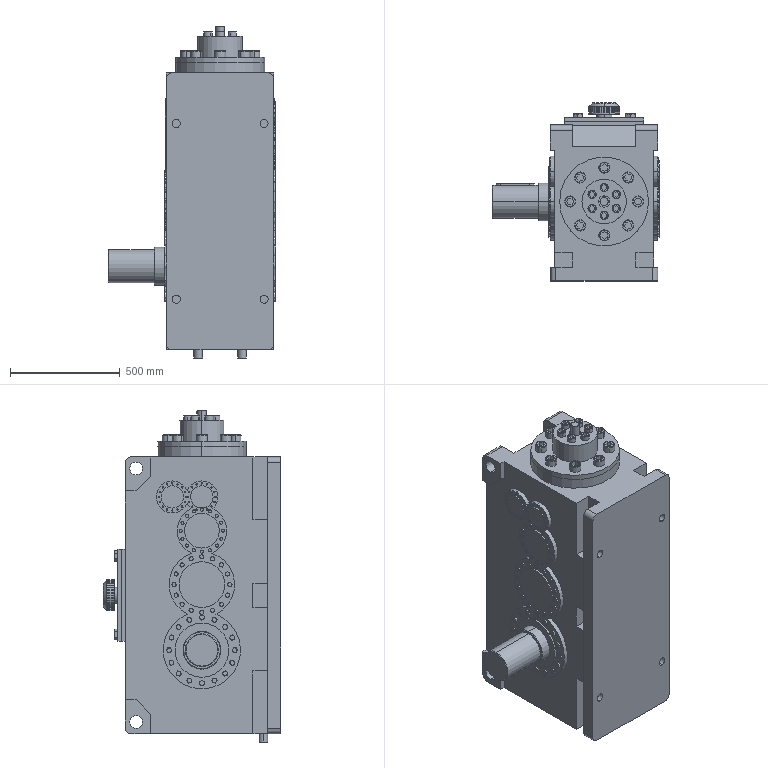Part | SolidWorks | features MBimport 1, Scale 1 | 5 solids | 2677 faces | box 763.452 x 810 x 1512 mm | volume 419343636 mm3 | plane 1498 | cone 988 | cylinder 161 | torus 30 | commonest cylinder face diameters 140 x36 50.625 x16 37.8 x12 145.6 x12 37 x8 57.857 x8